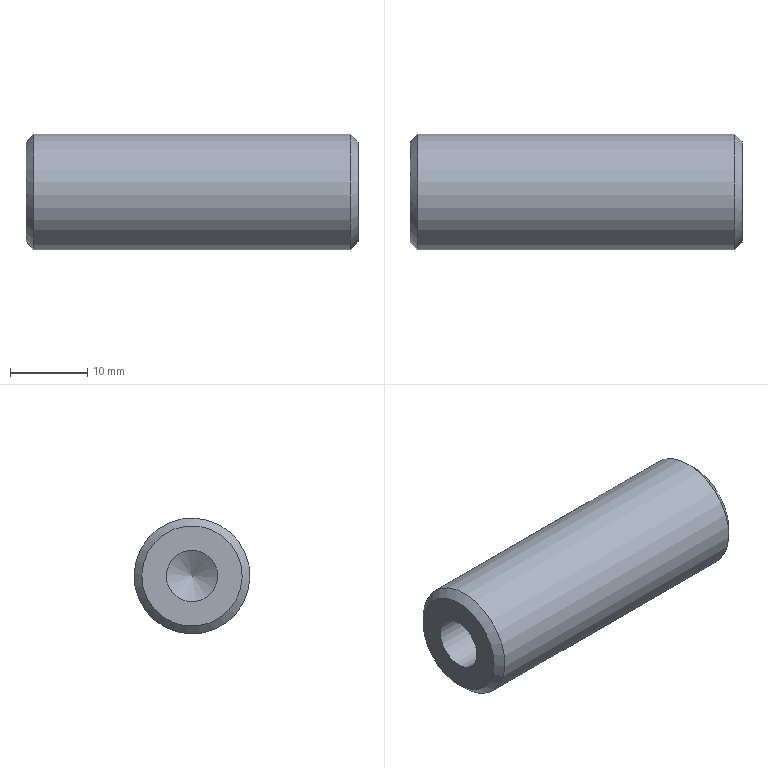Part | STEP file | SN10_013_002_PINO | 1 solid | 7 faces | box 43 x 15 x 15 mm | volume 6907 mm3 | cone 3 | plane 2 | cylinder 2 | commonest cylinder face diameters 6.647 x1 15 x1
STEP:
#1=CARTESIAN_POINT('',(0.,0.,0.));
#2=DIRECTION('',(0.,0.,1.));
#3=DIRECTION('',(1.,0.,0.));
#4=AXIS2_PLACEMENT_3D('',#1,#2,#3);
#5=CARTESIAN_POINT('',(38.,72.917,56.593));
#6=VERTEX_POINT('',#5);
#7=CARTESIAN_POINT('',(38.,70.,55.));
#8=DIRECTION('',(-1.,0.,0.));
#9=DIRECTION('',(0.,1.,0.));
#10=AXIS2_PLACEMENT_3D('',#7,#8,#9);
#11=CIRCLE('',#10,3.324);
#12=CARTESIAN_POINT('',(39.341,70.,55.));
#13=DIRECTION('',(-1.,0.,0.));
#14=DIRECTION('',(0.,0.8776,0.4794));
#15=AXIS2_PLACEMENT_3D('',#12,#13,#14);
#16=CONICAL_SURFACE('',#15,1.,1.047);
#17=CARTESIAN_POINT('',(-5.783,1.341));
#18=DIRECTION('',(1.,0.));
#19=VECTOR('',#18,1.);
#20=LINE('',#17,#19);
#21=(GEOMETRIC_REPRESENTATION_CONTEXT(2)PARAMETRIC_REPRESENTATION_CONTEXT()REPRESENTATION_CONTEXT('',''));
#22=DEFINITIONAL_REPRESENTATION('',(#20),#21);
#23=PCURVE('',#16,#22);
#24=CARTESIAN_POINT('',(20.1,70.,55.));
#25=DIRECTION('',(1.,0.,0.));
#26=DIRECTION('',(0.,0.8776,0.4794));
#27=AXIS2_PLACEMENT_3D('',#24,#25,#26);
#28=CYLINDRICAL_SURFACE('',#27,3.324);
#29=CARTESIAN_POINT('',(12.066,17.9));
#30=DIRECTION('',(-1.,0.));
#31=VECTOR('',#30,1.);
#32=LINE('',#29,#31);
#33=(GEOMETRIC_REPRESENTATION_CONTEXT(2)PARAMETRIC_REPRESENTATION_CONTEXT()REPRESENTATION_CONTEXT('',''));
#34=DEFINITIONAL_REPRESENTATION('',(#32),#33);
#35=PCURVE('',#28,#34);
#36=SURFACE_CURVE('',#11,(#23,#35),.PCURVE_S1.);
#37=EDGE_CURVE('',#6,#6,#36,.T.);
#38=ORIENTED_EDGE('',*,*,#37,.F.);
#39=CARTESIAN_POINT('',(39.919,70.,55.));
#40=VERTEX_POINT('',#39);
#41=CARTESIAN_POINT('',(39.919,70.,55.));
#42=CARTESIAN_POINT('',(38.,72.917,56.593));
#43=B_SPLINE_CURVE_WITH_KNOTS('',1,(#41,#42),.UNSPECIFIED.,.F.,.F.,(2,2),(-1.155,2.683),.PIECEWISE_BEZIER_KNOTS.);
#44=CARTESIAN_POINT('',(0.,0.));
#45=DIRECTION('',(0.,1.));
#46=VECTOR('',#45,1.);
#47=LINE('',#44,#46);
#48=(GEOMETRIC_REPRESENTATION_CONTEXT(2)PARAMETRIC_REPRESENTATION_CONTEXT()REPRESENTATION_CONTEXT('',''));
#49=DEFINITIONAL_REPRESENTATION('',(#47),#48);
#50=PCURVE('',#16,#49);
#51=CARTESIAN_POINT('',(6.283,0.));
#52=DIRECTION('',(0.,1.));
#53=VECTOR('',#52,1.);
#54=LINE('',#51,#53);
#55=(GEOMETRIC_REPRESENTATION_CONTEXT(2)PARAMETRIC_REPRESENTATION_CONTEXT()REPRESENTATION_CONTEXT('',''));
#56=DEFINITIONAL_REPRESENTATION('',(#54),#55);
#57=PCURVE('',#16,#56);
#58=SEAM_CURVE('',#43,(#50,#57),.PCURVE_S1.);
#59=EDGE_CURVE('',#40,#6,#58,.T.);
#60=ORIENTED_EDGE('',*,*,#59,.F.);
#61=ORIENTED_EDGE('',*,*,#59,.T.);
#62=EDGE_LOOP('',(#38,#60,#61));
#63=FACE_BOUND('',#62,.F.);
#64=ADVANCED_FACE('',(#63),#16,.F.);
#65=CARTESIAN_POINT('',(63.,64.296,51.884));
#66=VERTEX_POINT('',#65);
#67=CARTESIAN_POINT('',(63.,70.,55.));
#68=DIRECTION('',(1.,0.,0.));
#69=DIRECTION('',(0.,1.,0.));
#70=AXIS2_PLACEMENT_3D('',#67,#68,#69);
#71=CIRCLE('',#70,6.5);
#72=CARTESIAN_POINT('',(63.,77.5,55.));
#73=DIRECTION('',(1.,0.,0.));
#74=DIRECTION('',(0.,0.,-1.));
#75=AXIS2_PLACEMENT_3D('',#72,#73,#74);
#76=PLANE('',#75);
#77=CARTESIAN_POINT('',(0.,-7.5));
#78=DIRECTION('',(0.,1.));
#79=AXIS2_PLACEMENT_2D('',#77,#78);
#80=CIRCLE('',#79,6.5);
#81=(GEOMETRIC_REPRESENTATION_CONTEXT(2)PARAMETRIC_REPRESENTATION_CONTEXT()REPRESENTATION_CONTEXT('',''));
#82=DEFINITIONAL_REPRESENTATION('',(#80),#81);
#83=PCURVE('',#76,#82);
#84=CARTESIAN_POINT('',(68.5,70.,55.));
#85=DIRECTION('',(-1.,0.,0.));
#86=DIRECTION('',(0.,0.8776,0.4794));
#87=AXIS2_PLACEMENT_3D('',#84,#85,#86);
#88=CONICAL_SURFACE('',#87,1.,0.7854);
#89=CARTESIAN_POINT('',(13.066,5.5));
#90=DIRECTION('',(-1.,0.));
#91=VECTOR('',#90,1.);
#92=LINE('',#89,#91);
#93=(GEOMETRIC_REPRESENTATION_CONTEXT(2)PARAMETRIC_REPRESENTATION_CONTEXT()REPRESENTATION_CONTEXT('',''));
#94=DEFINITIONAL_REPRESENTATION('',(#92),#93);
#95=PCURVE('',#88,#94);
#96=SURFACE_CURVE('',#71,(#83,#95),.PCURVE_S1.);
#97=EDGE_CURVE('',#66,#66,#96,.T.);
#98=ORIENTED_EDGE('',*,*,#97,.T.);
#99=EDGE_LOOP('',(#98));
#100=FACE_BOUND('',#99,.T.);
#101=ADVANCED_FACE('',(#100),#76,.T.);
#102=ORIENTED_EDGE('',*,*,#97,.F.);
#103=CARTESIAN_POINT('',(62.,63.418,51.404));
#104=VERTEX_POINT('',#103);
#105=CARTESIAN_POINT('',(63.,64.296,51.884));
#106=CARTESIAN_POINT('',(62.,63.418,51.404));
#107=B_SPLINE_CURVE_WITH_KNOTS('',1,(#105,#106),.UNSPECIFIED.,.F.,.F.,(2,2),(7.778,9.192),.PIECEWISE_BEZIER_KNOTS.);
#108=CARTESIAN_POINT('',(9.425,0.));
#109=DIRECTION('',(0.,1.));
#110=VECTOR('',#109,1.);
#111=LINE('',#108,#110);
#112=(GEOMETRIC_REPRESENTATION_CONTEXT(2)PARAMETRIC_REPRESENTATION_CONTEXT()REPRESENTATION_CONTEXT('',''));
#113=DEFINITIONAL_REPRESENTATION('',(#111),#112);
#114=PCURVE('',#88,#113);
#115=CARTESIAN_POINT('',(3.142,0.));
#116=DIRECTION('',(0.,1.));
#117=VECTOR('',#116,1.);
#118=LINE('',#115,#117);
#119=(GEOMETRIC_REPRESENTATION_CONTEXT(2)PARAMETRIC_REPRESENTATION_CONTEXT()REPRESENTATION_CONTEXT('',''));
#120=DEFINITIONAL_REPRESENTATION('',(#118),#119);
#121=PCURVE('',#88,#120);
#122=SEAM_CURVE('',#107,(#114,#121),.PCURVE_S1.);
#123=EDGE_CURVE('',#66,#104,#122,.T.);
#124=ORIENTED_EDGE('',*,*,#123,.T.);
#125=CARTESIAN_POINT('',(62.,76.582,58.596));
#126=VERTEX_POINT('',#125);
#127=CARTESIAN_POINT('',(62.,70.,55.));
#128=DIRECTION('',(1.,0.,0.));
#129=DIRECTION('',(0.,1.,0.));
#130=AXIS2_PLACEMENT_3D('',#127,#128,#129);
#131=CIRCLE('',#130,7.5);
#132=CARTESIAN_POINT('',(13.066,6.5));
#133=DIRECTION('',(-1.,0.));
#134=VECTOR('',#133,1.);
#135=LINE('',#132,#134);
#136=(GEOMETRIC_REPRESENTATION_CONTEXT(2)PARAMETRIC_REPRESENTATION_CONTEXT()REPRESENTATION_CONTEXT('',''));
#137=DEFINITIONAL_REPRESENTATION('',(#135),#136);
#138=PCURVE('',#88,#137);
#139=CARTESIAN_POINT('',(41.5,70.,55.));
#140=DIRECTION('',(1.,0.,0.));
#141=DIRECTION('',(0.,0.8776,0.4794));
#142=AXIS2_PLACEMENT_3D('',#139,#140,#141);
#143=CYLINDRICAL_SURFACE('',#142,7.5);
#144=CARTESIAN_POINT('',(-0.5,20.5));
#145=DIRECTION('',(1.,0.));
#146=VECTOR('',#145,1.);
#147=LINE('',#144,#146);
#148=(GEOMETRIC_REPRESENTATION_CONTEXT(2)PARAMETRIC_REPRESENTATION_CONTEXT()REPRESENTATION_CONTEXT('',''));
#149=DEFINITIONAL_REPRESENTATION('',(#147),#148);
#150=PCURVE('',#143,#149);
#151=SURFACE_CURVE('',#131,(#138,#150),.PCURVE_S1.);
#152=EDGE_CURVE('',#104,#126,#151,.T.);
#153=ORIENTED_EDGE('',*,*,#152,.T.);
#154=CARTESIAN_POINT('',(62.,70.,55.));
#155=DIRECTION('',(1.,0.,0.));
#156=DIRECTION('',(0.,1.,0.));
#157=AXIS2_PLACEMENT_3D('',#154,#155,#156);
#158=CIRCLE('',#157,7.5);
#159=CARTESIAN_POINT('',(6.783,6.5));
#160=DIRECTION('',(-1.,0.));
#161=VECTOR('',#160,1.);
#162=LINE('',#159,#161);
#163=(GEOMETRIC_REPRESENTATION_CONTEXT(2)PARAMETRIC_REPRESENTATION_CONTEXT()REPRESENTATION_CONTEXT('',''));
#164=DEFINITIONAL_REPRESENTATION('',(#162),#163);
#165=PCURVE('',#88,#164);
#166=CARTESIAN_POINT('',(-0.5,20.5));
#167=DIRECTION('',(1.,0.));
#168=VECTOR('',#167,1.);
#169=LINE('',#166,#168);
#170=(GEOMETRIC_REPRESENTATION_CONTEXT(2)PARAMETRIC_REPRESENTATION_CONTEXT()REPRESENTATION_CONTEXT('',''));
#171=DEFINITIONAL_REPRESENTATION('',(#169),#170);
#172=PCURVE('',#143,#171);
#173=SURFACE_CURVE('',#158,(#165,#172),.PCURVE_S1.);
#174=EDGE_CURVE('',#126,#104,#173,.T.);
#175=ORIENTED_EDGE('',*,*,#174,.T.);
#176=ORIENTED_EDGE('',*,*,#123,.F.);
#177=EDGE_LOOP('',(#102,#124,#153,#175,#176));
#178=FACE_BOUND('',#177,.T.);
#179=ADVANCED_FACE('',(#178),#88,.T.);
#180=CARTESIAN_POINT('',(21.,76.582,58.596));
#181=VERTEX_POINT('',#180);
#182=CARTESIAN_POINT('',(21.,70.,55.));
#183=DIRECTION('',(1.,0.,0.));
#184=DIRECTION('',(0.,1.,0.));
#185=AXIS2_PLACEMENT_3D('',#182,#183,#184);
#186=CIRCLE('',#185,7.5);
#187=CARTESIAN_POINT('',(-0.5,-20.5));
#188=DIRECTION('',(1.,0.));
#189=VECTOR('',#188,1.);
#190=LINE('',#187,#189);
#191=(GEOMETRIC_REPRESENTATION_CONTEXT(2)PARAMETRIC_REPRESENTATION_CONTEXT()REPRESENTATION_CONTEXT('',''));
#192=DEFINITIONAL_REPRESENTATION('',(#190),#191);
#193=PCURVE('',#143,#192);
#194=CARTESIAN_POINT('',(14.5,70.,55.));
#195=DIRECTION('',(1.,0.,0.));
#196=DIRECTION('',(0.,0.8776,0.4794));
#197=AXIS2_PLACEMENT_3D('',#194,#195,#196);
#198=CONICAL_SURFACE('',#197,1.,0.7854);
#199=CARTESIAN_POINT('',(-0.5,6.5));
#200=DIRECTION('',(1.,0.));
#201=VECTOR('',#200,1.);
#202=LINE('',#199,#201);
#203=(GEOMETRIC_REPRESENTATION_CONTEXT(2)PARAMETRIC_REPRESENTATION_CONTEXT()REPRESENTATION_CONTEXT('',''));
#204=DEFINITIONAL_REPRESENTATION('',(#202),#203);
#205=PCURVE('',#198,#204);
#206=SURFACE_CURVE('',#186,(#193,#205),.PCURVE_S1.);
#207=EDGE_CURVE('',#181,#181,#206,.T.);
#208=ORIENTED_EDGE('',*,*,#207,.T.);
#209=CARTESIAN_POINT('',(21.,76.582,58.596));
#210=CARTESIAN_POINT('',(62.,76.582,58.596));
#211=B_SPLINE_CURVE_WITH_KNOTS('',1,(#209,#210),.UNSPECIFIED.,.F.,.F.,(2,2),(-20.5,20.5),.PIECEWISE_BEZIER_KNOTS.);
#212=CARTESIAN_POINT('',(6.283,0.));
#213=DIRECTION('',(0.,1.));
#214=VECTOR('',#213,1.);
#215=LINE('',#212,#214);
#216=(GEOMETRIC_REPRESENTATION_CONTEXT(2)PARAMETRIC_REPRESENTATION_CONTEXT()REPRESENTATION_CONTEXT('',''));
#217=DEFINITIONAL_REPRESENTATION('',(#215),#216);
#218=PCURVE('',#143,#217);
#219=CARTESIAN_POINT('',(0.,0.));
#220=DIRECTION('',(0.,1.));
#221=VECTOR('',#220,1.);
#222=LINE('',#219,#221);
#223=(GEOMETRIC_REPRESENTATION_CONTEXT(2)PARAMETRIC_REPRESENTATION_CONTEXT()REPRESENTATION_CONTEXT('',''));
#224=DEFINITIONAL_REPRESENTATION('',(#222),#223);
#225=PCURVE('',#143,#224);
#226=SEAM_CURVE('',#211,(#218,#225),.PCURVE_S1.);
#227=EDGE_CURVE('',#181,#126,#226,.T.);
#228=ORIENTED_EDGE('',*,*,#227,.T.);
#229=ORIENTED_EDGE('',*,*,#152,.F.);
#230=ORIENTED_EDGE('',*,*,#174,.F.);
#231=ORIENTED_EDGE('',*,*,#227,.F.);
#232=EDGE_LOOP('',(#208,#228,#229,#230,#231));
#233=FACE_BOUND('',#232,.T.);
#234=ADVANCED_FACE('',(#233),#143,.T.);
#235=ORIENTED_EDGE('',*,*,#207,.F.);
#236=CARTESIAN_POINT('',(20.,75.704,58.116));
#237=VERTEX_POINT('',#236);
#238=CARTESIAN_POINT('',(20.,75.704,58.116));
#239=CARTESIAN_POINT('',(21.,76.582,58.596));
#240=B_SPLINE_CURVE_WITH_KNOTS('',1,(#238,#239),.UNSPECIFIED.,.F.,.F.,(2,2),(7.778,9.192),.PIECEWISE_BEZIER_KNOTS.);
#241=CARTESIAN_POINT('',(0.,0.));
#242=DIRECTION('',(0.,1.));
#243=VECTOR('',#242,1.);
#244=LINE('',#241,#243);
#245=(GEOMETRIC_REPRESENTATION_CONTEXT(2)PARAMETRIC_REPRESENTATION_CONTEXT()REPRESENTATION_CONTEXT('',''));
#246=DEFINITIONAL_REPRESENTATION('',(#244),#245);
#247=PCURVE('',#198,#246);
#248=CARTESIAN_POINT('',(6.283,0.));
#249=DIRECTION('',(0.,1.));
#250=VECTOR('',#249,1.);
#251=LINE('',#248,#250);
#252=(GEOMETRIC_REPRESENTATION_CONTEXT(2)PARAMETRIC_REPRESENTATION_CONTEXT()REPRESENTATION_CONTEXT('',''));
#253=DEFINITIONAL_REPRESENTATION('',(#251),#252);
#254=PCURVE('',#198,#253);
#255=SEAM_CURVE('',#240,(#247,#254),.PCURVE_S1.);
#256=EDGE_CURVE('',#237,#181,#255,.T.);
#257=ORIENTED_EDGE('',*,*,#256,.F.);
#258=CARTESIAN_POINT('',(20.,64.296,51.884));
#259=VERTEX_POINT('',#258);
#260=CARTESIAN_POINT('',(20.,70.,55.));
#261=DIRECTION('',(1.,0.,0.));
#262=DIRECTION('',(0.,1.,0.));
#263=AXIS2_PLACEMENT_3D('',#260,#261,#262);
#264=CIRCLE('',#263,6.5);
#265=CARTESIAN_POINT('',(-0.5,5.5));
#266=DIRECTION('',(1.,0.));
#267=VECTOR('',#266,1.);
#268=LINE('',#265,#267);
#269=(GEOMETRIC_REPRESENTATION_CONTEXT(2)PARAMETRIC_REPRESENTATION_CONTEXT()REPRESENTATION_CONTEXT('',''));
#270=DEFINITIONAL_REPRESENTATION('',(#268),#269);
#271=PCURVE('',#198,#270);
#272=CARTESIAN_POINT('',(20.,70.,55.));
#273=DIRECTION('',(1.,0.,0.));
#274=DIRECTION('',(0.,0.,-1.));
#275=AXIS2_PLACEMENT_3D('',#272,#273,#274);
#276=PLANE('',#275);
#277=CARTESIAN_POINT('',(0.,0.));
#278=DIRECTION('',(0.,1.));
#279=AXIS2_PLACEMENT_2D('',#277,#278);
#280=CIRCLE('',#279,6.5);
#281=(GEOMETRIC_REPRESENTATION_CONTEXT(2)PARAMETRIC_REPRESENTATION_CONTEXT()REPRESENTATION_CONTEXT('',''));
#282=DEFINITIONAL_REPRESENTATION('',(#280),#281);
#283=PCURVE('',#276,#282);
#284=SURFACE_CURVE('',#264,(#271,#283),.PCURVE_S1.);
#285=EDGE_CURVE('',#237,#259,#284,.T.);
#286=ORIENTED_EDGE('',*,*,#285,.T.);
#287=CARTESIAN_POINT('',(20.,70.,55.));
#288=DIRECTION('',(1.,0.,0.));
#289=DIRECTION('',(0.,1.,0.));
#290=AXIS2_PLACEMENT_3D('',#287,#288,#289);
#291=CIRCLE('',#290,6.5);
#292=CARTESIAN_POINT('',(-0.5,5.5));
#293=DIRECTION('',(1.,0.));
#294=VECTOR('',#293,1.);
#295=LINE('',#292,#294);
#296=(GEOMETRIC_REPRESENTATION_CONTEXT(2)PARAMETRIC_REPRESENTATION_CONTEXT()REPRESENTATION_CONTEXT('',''));
#297=DEFINITIONAL_REPRESENTATION('',(#295),#296);
#298=PCURVE('',#198,#297);
#299=CARTESIAN_POINT('',(0.,0.));
#300=DIRECTION('',(0.,1.));
#301=AXIS2_PLACEMENT_2D('',#299,#300);
#302=CIRCLE('',#301,6.5);
#303=(GEOMETRIC_REPRESENTATION_CONTEXT(2)PARAMETRIC_REPRESENTATION_CONTEXT()REPRESENTATION_CONTEXT('',''));
#304=DEFINITIONAL_REPRESENTATION('',(#302),#303);
#305=PCURVE('',#276,#304);
#306=SURFACE_CURVE('',#291,(#298,#305),.PCURVE_S1.);
#307=EDGE_CURVE('',#259,#237,#306,.T.);
#308=ORIENTED_EDGE('',*,*,#307,.T.);
#309=ORIENTED_EDGE('',*,*,#256,.T.);
#310=EDGE_LOOP('',(#235,#257,#286,#308,#309));
#311=FACE_BOUND('',#310,.T.);
#312=ADVANCED_FACE('',(#311),#198,.T.);
#313=ORIENTED_EDGE('',*,*,#307,.F.);
#314=ORIENTED_EDGE('',*,*,#285,.F.);
#315=EDGE_LOOP('',(#313,#314));
#316=FACE_BOUND('',#315,.T.);
#317=CARTESIAN_POINT('',(20.,72.917,56.593));
#318=VERTEX_POINT('',#317);
#319=CARTESIAN_POINT('',(20.,70.,55.));
#320=DIRECTION('',(1.,0.,0.));
#321=DIRECTION('',(0.,1.,0.));
#322=AXIS2_PLACEMENT_3D('',#319,#320,#321);
#323=CIRCLE('',#322,3.324);
#324=CARTESIAN_POINT('',(0.,0.));
#325=DIRECTION('',(0.,1.));
#326=AXIS2_PLACEMENT_2D('',#324,#325);
#327=CIRCLE('',#326,3.324);
#328=(GEOMETRIC_REPRESENTATION_CONTEXT(2)PARAMETRIC_REPRESENTATION_CONTEXT()REPRESENTATION_CONTEXT('',''));
#329=DEFINITIONAL_REPRESENTATION('',(#327),#328);
#330=PCURVE('',#276,#329);
#331=CARTESIAN_POINT('',(-0.5,-0.1));
#332=DIRECTION('',(1.,0.));
#333=VECTOR('',#332,1.);
#334=LINE('',#331,#333);
#335=(GEOMETRIC_REPRESENTATION_CONTEXT(2)PARAMETRIC_REPRESENTATION_CONTEXT()REPRESENTATION_CONTEXT('',''));
#336=DEFINITIONAL_REPRESENTATION('',(#334),#335);
#337=PCURVE('',#28,#336);
#338=SURFACE_CURVE('',#323,(#330,#337),.PCURVE_S1.);
#339=EDGE_CURVE('',#318,#318,#338,.T.);
#340=ORIENTED_EDGE('',*,*,#339,.T.);
#341=EDGE_LOOP('',(#340));
#342=FACE_BOUND('',#341,.T.);
#343=ADVANCED_FACE('',(#316,#342),#276,.F.);
#344=ORIENTED_EDGE('',*,*,#339,.T.);
#345=CARTESIAN_POINT('',(20.,72.917,56.593));
#346=CARTESIAN_POINT('',(38.,72.917,56.593));
#347=B_SPLINE_CURVE_WITH_KNOTS('',1,(#345,#346),.UNSPECIFIED.,.F.,.F.,(2,2),(-0.1,17.9),.PIECEWISE_BEZIER_KNOTS.);
#348=CARTESIAN_POINT('',(6.283,0.));
#349=DIRECTION('',(0.,1.));
#350=VECTOR('',#349,1.);
#351=LINE('',#348,#350);
#352=(GEOMETRIC_REPRESENTATION_CONTEXT(2)PARAMETRIC_REPRESENTATION_CONTEXT()REPRESENTATION_CONTEXT('',''));
#353=DEFINITIONAL_REPRESENTATION('',(#351),#352);
#354=PCURVE('',#28,#353);
#355=CARTESIAN_POINT('',(0.,0.));
#356=DIRECTION('',(0.,1.));
#357=VECTOR('',#356,1.);
#358=LINE('',#355,#357);
#359=(GEOMETRIC_REPRESENTATION_CONTEXT(2)PARAMETRIC_REPRESENTATION_CONTEXT()REPRESENTATION_CONTEXT('',''));
#360=DEFINITIONAL_REPRESENTATION('',(#358),#359);
#361=PCURVE('',#28,#360);
#362=SEAM_CURVE('',#347,(#354,#361),.PCURVE_S1.);
#363=EDGE_CURVE('',#318,#6,#362,.T.);
#364=ORIENTED_EDGE('',*,*,#363,.T.);
#365=ORIENTED_EDGE('',*,*,#37,.T.);
#366=ORIENTED_EDGE('',*,*,#363,.F.);
#367=EDGE_LOOP('',(#344,#364,#365,#366));
#368=FACE_BOUND('',#367,.F.);
#369=ADVANCED_FACE('',(#368),#28,.F.);
#370=CLOSED_SHELL('',(#64,#101,#179,#234,#312,#343,#369));
#371=MANIFOLD_SOLID_BREP('',#370);
#372=(LENGTH_UNIT()NAMED_UNIT(*)SI_UNIT(.MILLI.,.METRE.));
#373=UNCERTAINTY_MEASURE_WITH_UNIT(LENGTH_MEASURE(0.00001),#372,'','');
#374=(NAMED_UNIT(*)PLANE_ANGLE_UNIT()SI_UNIT($,.RADIAN.));
#375=(NAMED_UNIT(*)SI_UNIT($,.STERADIAN.)SOLID_ANGLE_UNIT());
#376=(GEOMETRIC_REPRESENTATION_CONTEXT(3)GLOBAL_UNCERTAINTY_ASSIGNED_CONTEXT((#373))GLOBAL_UNIT_ASSIGNED_CONTEXT((#372,#374,#375))REPRESENTATION_CONTEXT('',''));
#377=ADVANCED_BREP_SHAPE_REPRESENTATION('',(#4,#371),#376);